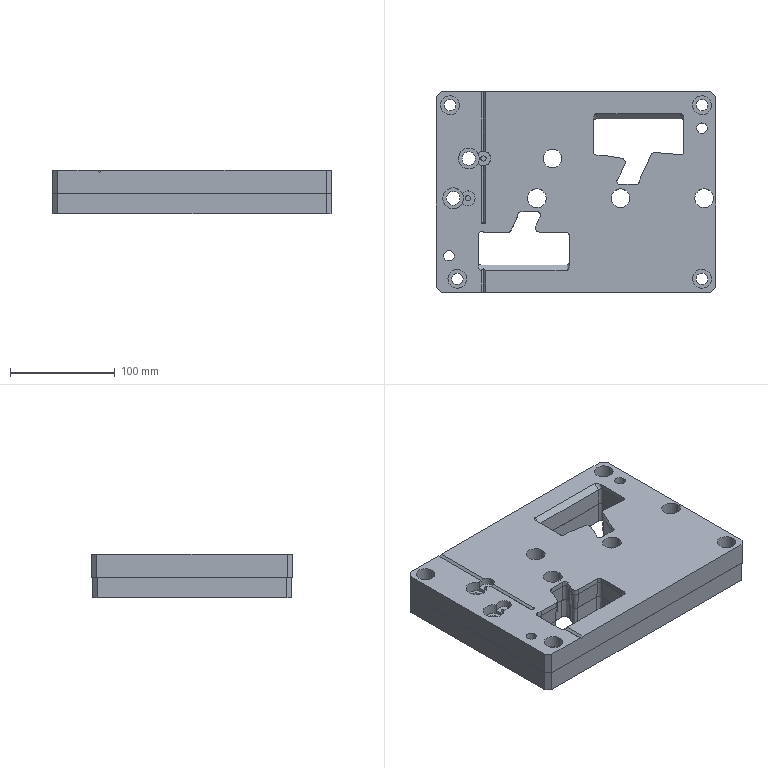Part | CATIA | 2 solids | 225 faces | box 267 x 192 x 42 mm | volume 1738037 mm3 | cylinder 80 | plane 66 | other 54 | spline 25 | commonest cylinder face diameters 18 x16 11 x12 6 x8 12 x8 22 x8 5 x4